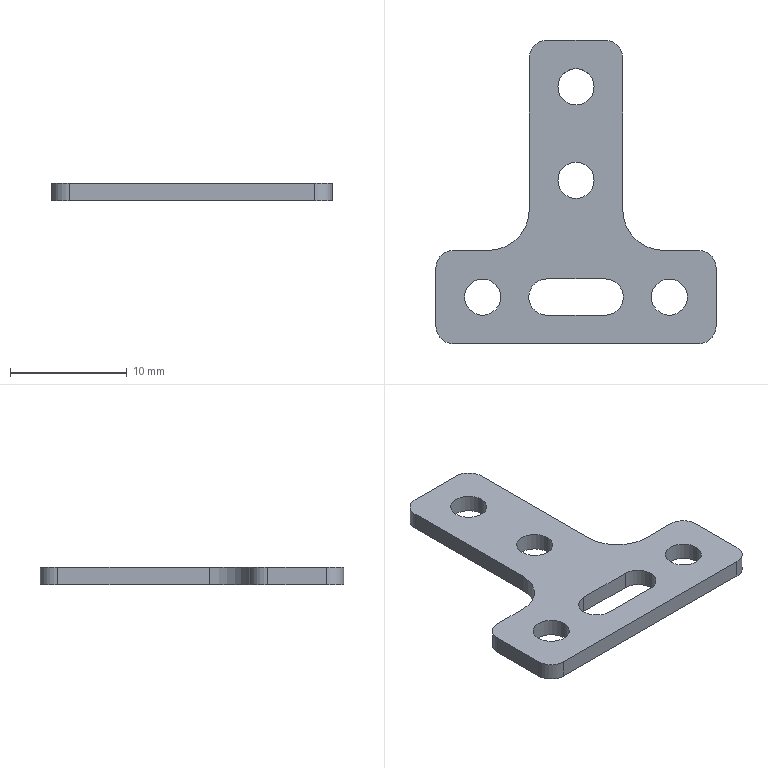Part | SolidWorks | features Fillet 2, Extrusion 1 | 1 solid | 31 faces | box 24 x 26 x 1.5 mm | volume 427.683 mm3 | cylinder 19 | plane 12 | commonest cylinder face diameters 3.1 x11 3 x6 7 x2
STEP:
#1=CARTESIAN_POINT('',(-6.45,0.,1.5));
#2=VERTEX_POINT('',#1);
#3=CARTESIAN_POINT('',(-9.55,0.,1.5));
#4=VERTEX_POINT('',#3);
#5=CARTESIAN_POINT('',(-8.,0.,1.5));
#6=DIRECTION('',(0.,0.,-1.));
#7=DIRECTION('',(1.,0.,0.));
#8=AXIS2_PLACEMENT_3D('',#5,#6,#7);
#9=CIRCLE('',#8,1.55);
#10=EDGE_CURVE('',#2,#4,#9,.T.);
#11=ORIENTED_EDGE('',*,*,#10,.F.);
#12=CARTESIAN_POINT('',(-6.45,0.,0.));
#13=VERTEX_POINT('',#12);
#14=CARTESIAN_POINT('',(-6.45,0.,1.5));
#15=DIRECTION('',(0.,0.,-1.));
#16=VECTOR('',#15,1000.);
#17=LINE('',#14,#16);
#18=EDGE_CURVE('',#2,#13,#17,.T.);
#19=ORIENTED_EDGE('',*,*,#18,.T.);
#20=CARTESIAN_POINT('',(-9.55,0.,0.));
#21=VERTEX_POINT('',#20);
#22=CARTESIAN_POINT('',(-8.,0.,0.));
#23=DIRECTION('',(0.,0.,-1.));
#24=DIRECTION('',(1.,0.,0.));
#25=AXIS2_PLACEMENT_3D('',#22,#23,#24);
#26=CIRCLE('',#25,1.55);
#27=EDGE_CURVE('',#13,#21,#26,.T.);
#28=ORIENTED_EDGE('',*,*,#27,.T.);
#29=CARTESIAN_POINT('',(-9.55,0.,1.5));
#30=DIRECTION('',(0.,0.,-1.));
#31=VECTOR('',#30,1000.);
#32=LINE('',#29,#31);
#33=EDGE_CURVE('',#4,#21,#32,.T.);
#34=ORIENTED_EDGE('',*,*,#33,.F.);
#35=EDGE_LOOP('',(#11,#19,#28,#34));
#36=FACE_OUTER_BOUND('',#35,.T.);
#37=CARTESIAN_POINT('',(-8.,0.,1.5));
#38=DIRECTION('',(0.,0.,-1.));
#39=DIRECTION('',(-1.,0.,0.));
#40=AXIS2_PLACEMENT_3D('',#37,#38,#39);
#41=CYLINDRICAL_SURFACE('',#40,1.55);
#42=ADVANCED_FACE('',(#36),#41,.F.);
#43=CARTESIAN_POINT('',(-1.55,18.,1.5));
#44=VERTEX_POINT('',#43);
#45=CARTESIAN_POINT('',(1.55,18.,1.5));
#46=VERTEX_POINT('',#45);
#47=CARTESIAN_POINT('',(0.,18.,1.5));
#48=DIRECTION('',(0.,0.,1.));
#49=DIRECTION('',(1.,0.,0.));
#50=AXIS2_PLACEMENT_3D('',#47,#48,#49);
#51=CIRCLE('',#50,1.55);
#52=EDGE_CURVE('',#44,#46,#51,.T.);
#53=ORIENTED_EDGE('',*,*,#52,.T.);
#54=CARTESIAN_POINT('',(1.55,18.,0.));
#55=VERTEX_POINT('',#54);
#56=CARTESIAN_POINT('',(1.55,18.,1.5));
#57=DIRECTION('',(0.,0.,-1.));
#58=VECTOR('',#57,1000.);
#59=LINE('',#56,#58);
#60=EDGE_CURVE('',#46,#55,#59,.T.);
#61=ORIENTED_EDGE('',*,*,#60,.T.);
#62=CARTESIAN_POINT('',(-1.55,18.,0.));
#63=VERTEX_POINT('',#62);
#64=CARTESIAN_POINT('',(0.,18.,0.));
#65=DIRECTION('',(0.,0.,1.));
#66=DIRECTION('',(1.,0.,0.));
#67=AXIS2_PLACEMENT_3D('',#64,#65,#66);
#68=CIRCLE('',#67,1.55);
#69=EDGE_CURVE('',#63,#55,#68,.T.);
#70=ORIENTED_EDGE('',*,*,#69,.F.);
#71=CARTESIAN_POINT('',(-1.55,18.,1.5));
#72=DIRECTION('',(0.,0.,-1.));
#73=VECTOR('',#72,1000.);
#74=LINE('',#71,#73);
#75=EDGE_CURVE('',#44,#63,#74,.T.);
#76=ORIENTED_EDGE('',*,*,#75,.F.);
#77=EDGE_LOOP('',(#53,#61,#70,#76));
#78=FACE_OUTER_BOUND('',#77,.T.);
#79=CARTESIAN_POINT('',(0.,18.,1.5));
#80=DIRECTION('',(0.,0.,-1.));
#81=DIRECTION('',(-1.,0.,0.));
#82=AXIS2_PLACEMENT_3D('',#79,#80,#81);
#83=CYLINDRICAL_SURFACE('',#82,1.55);
#84=ADVANCED_FACE('',(#78),#83,.F.);
#85=CARTESIAN_POINT('',(-1.55,10.,1.5));
#86=VERTEX_POINT('',#85);
#87=CARTESIAN_POINT('',(1.55,10.,1.5));
#88=VERTEX_POINT('',#87);
#89=CARTESIAN_POINT('',(0.,10.,1.5));
#90=DIRECTION('',(0.,0.,1.));
#91=DIRECTION('',(1.,0.,0.));
#92=AXIS2_PLACEMENT_3D('',#89,#90,#91);
#93=CIRCLE('',#92,1.55);
#94=EDGE_CURVE('',#86,#88,#93,.T.);
#95=ORIENTED_EDGE('',*,*,#94,.T.);
#96=CARTESIAN_POINT('',(1.55,10.,0.));
#97=VERTEX_POINT('',#96);
#98=CARTESIAN_POINT('',(1.55,10.,1.5));
#99=DIRECTION('',(0.,0.,-1.));
#100=VECTOR('',#99,1000.);
#101=LINE('',#98,#100);
#102=EDGE_CURVE('',#88,#97,#101,.T.);
#103=ORIENTED_EDGE('',*,*,#102,.T.);
#104=CARTESIAN_POINT('',(-1.55,10.,0.));
#105=VERTEX_POINT('',#104);
#106=CARTESIAN_POINT('',(0.,10.,0.));
#107=DIRECTION('',(0.,0.,1.));
#108=DIRECTION('',(1.,0.,0.));
#109=AXIS2_PLACEMENT_3D('',#106,#107,#108);
#110=CIRCLE('',#109,1.55);
#111=EDGE_CURVE('',#105,#97,#110,.T.);
#112=ORIENTED_EDGE('',*,*,#111,.F.);
#113=CARTESIAN_POINT('',(-1.55,10.,1.5));
#114=DIRECTION('',(0.,0.,-1.));
#115=VECTOR('',#114,1000.);
#116=LINE('',#113,#115);
#117=EDGE_CURVE('',#86,#105,#116,.T.);
#118=ORIENTED_EDGE('',*,*,#117,.F.);
#119=EDGE_LOOP('',(#95,#103,#112,#118));
#120=FACE_OUTER_BOUND('',#119,.T.);
#121=CARTESIAN_POINT('',(0.,10.,1.5));
#122=DIRECTION('',(0.,0.,-1.));
#123=DIRECTION('',(-1.,0.,0.));
#124=AXIS2_PLACEMENT_3D('',#121,#122,#123);
#125=CYLINDRICAL_SURFACE('',#124,1.55);
#126=ADVANCED_FACE('',(#120),#125,.F.);
#127=CARTESIAN_POINT('',(6.45,0.,1.5));
#128=VERTEX_POINT('',#127);
#129=CARTESIAN_POINT('',(9.55,0.,1.5));
#130=VERTEX_POINT('',#129);
#131=CARTESIAN_POINT('',(8.,0.,1.5));
#132=DIRECTION('',(0.,0.,1.));
#133=DIRECTION('',(1.,0.,0.));
#134=AXIS2_PLACEMENT_3D('',#131,#132,#133);
#135=CIRCLE('',#134,1.55);
#136=EDGE_CURVE('',#128,#130,#135,.T.);
#137=ORIENTED_EDGE('',*,*,#136,.T.);
#138=CARTESIAN_POINT('',(9.55,0.,0.));
#139=VERTEX_POINT('',#138);
#140=CARTESIAN_POINT('',(9.55,0.,1.5));
#141=DIRECTION('',(0.,0.,-1.));
#142=VECTOR('',#141,1000.);
#143=LINE('',#140,#142);
#144=EDGE_CURVE('',#130,#139,#143,.T.);
#145=ORIENTED_EDGE('',*,*,#144,.T.);
#146=CARTESIAN_POINT('',(6.45,0.,0.));
#147=VERTEX_POINT('',#146);
#148=CARTESIAN_POINT('',(8.,0.,0.));
#149=DIRECTION('',(0.,0.,1.));
#150=DIRECTION('',(1.,0.,0.));
#151=AXIS2_PLACEMENT_3D('',#148,#149,#150);
#152=CIRCLE('',#151,1.55);
#153=EDGE_CURVE('',#147,#139,#152,.T.);
#154=ORIENTED_EDGE('',*,*,#153,.F.);
#155=CARTESIAN_POINT('',(6.45,0.,1.5));
#156=DIRECTION('',(0.,0.,-1.));
#157=VECTOR('',#156,1000.);
#158=LINE('',#155,#157);
#159=EDGE_CURVE('',#128,#147,#158,.T.);
#160=ORIENTED_EDGE('',*,*,#159,.F.);
#161=EDGE_LOOP('',(#137,#145,#154,#160));
#162=FACE_OUTER_BOUND('',#161,.T.);
#163=CARTESIAN_POINT('',(8.,0.,1.5));
#164=DIRECTION('',(0.,0.,-1.));
#165=DIRECTION('',(-1.,0.,0.));
#166=AXIS2_PLACEMENT_3D('',#163,#164,#165);
#167=CYLINDRICAL_SURFACE('',#166,1.55);
#168=ADVANCED_FACE('',(#162),#167,.F.);
#169=CARTESIAN_POINT('',(-2.5,1.55,1.5));
#170=VERTEX_POINT('',#169);
#171=CARTESIAN_POINT('',(-4.05,0.,1.5));
#172=VERTEX_POINT('',#171);
#173=CARTESIAN_POINT('',(-2.5,0.,1.5));
#174=DIRECTION('',(0.,0.,1.));
#175=DIRECTION('',(1.,0.,0.));
#176=AXIS2_PLACEMENT_3D('',#173,#174,#175);
#177=CIRCLE('',#176,1.55);
#178=EDGE_CURVE('',#170,#172,#177,.T.);
#179=ORIENTED_EDGE('',*,*,#178,.T.);
#180=CARTESIAN_POINT('',(-4.05,0.,0.));
#181=VERTEX_POINT('',#180);
#182=CARTESIAN_POINT('',(-4.05,0.,1.5));
#183=DIRECTION('',(0.,0.,-1.));
#184=VECTOR('',#183,1000.);
#185=LINE('',#182,#184);
#186=EDGE_CURVE('',#172,#181,#185,.T.);
#187=ORIENTED_EDGE('',*,*,#186,.T.);
#188=CARTESIAN_POINT('',(-2.5,1.55,0.));
#189=VERTEX_POINT('',#188);
#190=CARTESIAN_POINT('',(-2.5,0.,0.));
#191=DIRECTION('',(0.,0.,1.));
#192=DIRECTION('',(1.,0.,0.));
#193=AXIS2_PLACEMENT_3D('',#190,#191,#192);
#194=CIRCLE('',#193,1.55);
#195=EDGE_CURVE('',#189,#181,#194,.T.);
#196=ORIENTED_EDGE('',*,*,#195,.F.);
#197=CARTESIAN_POINT('',(-2.5,1.55,1.5));
#198=DIRECTION('',(0.,0.,-1.));
#199=VECTOR('',#198,1000.);
#200=LINE('',#197,#199);
#201=EDGE_CURVE('',#170,#189,#200,.T.);
#202=ORIENTED_EDGE('',*,*,#201,.F.);
#203=EDGE_LOOP('',(#179,#187,#196,#202));
#204=FACE_OUTER_BOUND('',#203,.T.);
#205=CARTESIAN_POINT('',(-2.5,0.,1.5));
#206=DIRECTION('',(0.,0.,-1.));
#207=DIRECTION('',(-1.,0.,0.));
#208=AXIS2_PLACEMENT_3D('',#205,#206,#207);
#209=CYLINDRICAL_SURFACE('',#208,1.55);
#210=ADVANCED_FACE('',(#204),#209,.F.);
#211=CARTESIAN_POINT('',(4.,20.5,1.5));
#212=VERTEX_POINT('',#211);
#213=CARTESIAN_POINT('',(4.,7.5,1.5));
#214=VERTEX_POINT('',#213);
#215=CARTESIAN_POINT('',(4.,0.,1.5));
#216=DIRECTION('',(0.,-1.,0.));
#217=VECTOR('',#216,1000.);
#218=LINE('',#215,#217);
#219=EDGE_CURVE('',#212,#214,#218,.T.);
#220=ORIENTED_EDGE('',*,*,#219,.T.);
#221=CARTESIAN_POINT('',(4.,7.5,0.));
#222=VERTEX_POINT('',#221);
#223=CARTESIAN_POINT('',(4.,7.5,0.));
#224=DIRECTION('',(0.,0.,-1.));
#225=VECTOR('',#224,1000.);
#226=LINE('',#223,#225);
#227=EDGE_CURVE('',#214,#222,#226,.T.);
#228=ORIENTED_EDGE('',*,*,#227,.T.);
#229=CARTESIAN_POINT('',(4.,20.5,0.));
#230=VERTEX_POINT('',#229);
#231=CARTESIAN_POINT('',(4.,0.,0.));
#232=DIRECTION('',(0.,-1.,0.));
#233=VECTOR('',#232,1000.);
#234=LINE('',#231,#233);
#235=EDGE_CURVE('',#230,#222,#234,.T.);
#236=ORIENTED_EDGE('',*,*,#235,.F.);
#237=CARTESIAN_POINT('',(4.,20.5,1.5));
#238=DIRECTION('',(0.,0.,1.));
#239=VECTOR('',#238,1000.);
#240=LINE('',#237,#239);
#241=EDGE_CURVE('',#230,#212,#240,.T.);
#242=ORIENTED_EDGE('',*,*,#241,.T.);
#243=EDGE_LOOP('',(#220,#228,#236,#242));
#244=FACE_OUTER_BOUND('',#243,.T.);
#245=CARTESIAN_POINT('',(4.,0.,1.5));
#246=DIRECTION('',(1.,0.,0.));
#247=DIRECTION('',(0.,1.,0.));
#248=AXIS2_PLACEMENT_3D('',#245,#246,#247);
#249=PLANE('',#248);
#250=ADVANCED_FACE('',(#244),#249,.T.);
#251=CARTESIAN_POINT('',(2.5,22.,1.5));
#252=VERTEX_POINT('',#251);
#253=CARTESIAN_POINT('',(-2.5,22.,1.5));
#254=VERTEX_POINT('',#253);
#255=CARTESIAN_POINT('',(0.,22.,1.5));
#256=DIRECTION('',(-1.,0.,0.));
#257=VECTOR('',#256,1000.);
#258=LINE('',#255,#257);
#259=EDGE_CURVE('',#252,#254,#258,.T.);
#260=ORIENTED_EDGE('',*,*,#259,.F.);
#261=CARTESIAN_POINT('',(2.5,22.,0.));
#262=VERTEX_POINT('',#261);
#263=CARTESIAN_POINT('',(2.5,22.,0.));
#264=DIRECTION('',(0.,0.,-1.));
#265=VECTOR('',#264,1000.);
#266=LINE('',#263,#265);
#267=EDGE_CURVE('',#252,#262,#266,.T.);
#268=ORIENTED_EDGE('',*,*,#267,.T.);
#269=CARTESIAN_POINT('',(-2.5,22.,0.));
#270=VERTEX_POINT('',#269);
#271=CARTESIAN_POINT('',(0.,22.,0.));
#272=DIRECTION('',(-1.,0.,0.));
#273=VECTOR('',#272,1000.);
#274=LINE('',#271,#273);
#275=EDGE_CURVE('',#262,#270,#274,.T.);
#276=ORIENTED_EDGE('',*,*,#275,.T.);
#277=CARTESIAN_POINT('',(-2.5,22.,1.5));
#278=DIRECTION('',(0.,0.,1.));
#279=VECTOR('',#278,1000.);
#280=LINE('',#277,#279);
#281=EDGE_CURVE('',#270,#254,#280,.T.);
#282=ORIENTED_EDGE('',*,*,#281,.T.);
#283=EDGE_LOOP('',(#260,#268,#276,#282));
#284=FACE_OUTER_BOUND('',#283,.T.);
#285=CARTESIAN_POINT('',(0.,22.,1.5));
#286=DIRECTION('',(0.,-1.,0.));
#287=DIRECTION('',(0.,0.,-1.));
#288=AXIS2_PLACEMENT_3D('',#285,#286,#287);
#289=PLANE('',#288);
#290=ADVANCED_FACE('',(#284),#289,.F.);
#291=CARTESIAN_POINT('',(-4.,20.5,0.));
#292=VERTEX_POINT('',#291);
#293=CARTESIAN_POINT('',(-4.,7.5,0.));
#294=VERTEX_POINT('',#293);
#295=CARTESIAN_POINT('',(-4.,0.,0.));
#296=DIRECTION('',(0.,-1.,0.));
#297=VECTOR('',#296,1000.);
#298=LINE('',#295,#297);
#299=EDGE_CURVE('',#292,#294,#298,.T.);
#300=ORIENTED_EDGE('',*,*,#299,.T.);
#301=CARTESIAN_POINT('',(-4.,7.5,1.5));
#302=VERTEX_POINT('',#301);
#303=CARTESIAN_POINT('',(-4.,7.5,1.5));
#304=DIRECTION('',(0.,0.,1.));
#305=VECTOR('',#304,1000.);
#306=LINE('',#303,#305);
#307=EDGE_CURVE('',#294,#302,#306,.T.);
#308=ORIENTED_EDGE('',*,*,#307,.T.);
#309=CARTESIAN_POINT('',(-4.,20.5,1.5));
#310=VERTEX_POINT('',#309);
#311=CARTESIAN_POINT('',(-4.,0.,1.5));
#312=DIRECTION('',(0.,-1.,0.));
#313=VECTOR('',#312,1000.);
#314=LINE('',#311,#313);
#315=EDGE_CURVE('',#310,#302,#314,.T.);
#316=ORIENTED_EDGE('',*,*,#315,.F.);
#317=CARTESIAN_POINT('',(-4.,20.5,1.5));
#318=DIRECTION('',(0.,0.,-1.));
#319=VECTOR('',#318,1000.);
#320=LINE('',#317,#319);
#321=EDGE_CURVE('',#310,#292,#320,.T.);
#322=ORIENTED_EDGE('',*,*,#321,.T.);
#323=EDGE_LOOP('',(#300,#308,#316,#322));
#324=FACE_OUTER_BOUND('',#323,.T.);
#325=CARTESIAN_POINT('',(-4.,0.,1.5));
#326=DIRECTION('',(1.,0.,0.));
#327=DIRECTION('',(0.,1.,0.));
#328=AXIS2_PLACEMENT_3D('',#325,#326,#327);
#329=PLANE('',#328);
#330=ADVANCED_FACE('',(#324),#329,.F.);
#331=CARTESIAN_POINT('',(-7.5,4.,1.5));
#332=VERTEX_POINT('',#331);
#333=CARTESIAN_POINT('',(-10.5,4.,1.5));
#334=VERTEX_POINT('',#333);
#335=CARTESIAN_POINT('',(0.,4.,1.5));
#336=DIRECTION('',(-1.,0.,0.));
#337=VECTOR('',#336,1000.);
#338=LINE('',#335,#337);
#339=EDGE_CURVE('',#332,#334,#338,.T.);
#340=ORIENTED_EDGE('',*,*,#339,.F.);
#341=CARTESIAN_POINT('',(-7.5,4.,0.));
#342=VERTEX_POINT('',#341);
#343=CARTESIAN_POINT('',(-7.5,4.,0.));
#344=DIRECTION('',(0.,0.,-1.));
#345=VECTOR('',#344,1000.);
#346=LINE('',#343,#345);
#347=EDGE_CURVE('',#332,#342,#346,.T.);
#348=ORIENTED_EDGE('',*,*,#347,.T.);
#349=CARTESIAN_POINT('',(-10.5,4.,0.));
#350=VERTEX_POINT('',#349);
#351=CARTESIAN_POINT('',(0.,4.,0.));
#352=DIRECTION('',(-1.,0.,0.));
#353=VECTOR('',#352,1000.);
#354=LINE('',#351,#353);
#355=EDGE_CURVE('',#342,#350,#354,.T.);
#356=ORIENTED_EDGE('',*,*,#355,.T.);
#357=CARTESIAN_POINT('',(-10.5,4.,1.5));
#358=DIRECTION('',(0.,0.,1.));
#359=VECTOR('',#358,1000.);
#360=LINE('',#357,#359);
#361=EDGE_CURVE('',#350,#334,#360,.T.);
#362=ORIENTED_EDGE('',*,*,#361,.T.);
#363=EDGE_LOOP('',(#340,#348,#356,#362));
#364=FACE_OUTER_BOUND('',#363,.T.);
#365=CARTESIAN_POINT('',(0.,4.,1.5));
#366=DIRECTION('',(0.,-1.,0.));
#367=DIRECTION('',(1.,0.,0.));
#368=AXIS2_PLACEMENT_3D('',#365,#366,#367);
#369=PLANE('',#368);
#370=ADVANCED_FACE('',(#364),#369,.F.);
#371=CARTESIAN_POINT('',(-12.,2.5,0.));
#372=VERTEX_POINT('',#371);
#373=CARTESIAN_POINT('',(-12.,-2.5,0.));
#374=VERTEX_POINT('',#373);
#375=CARTESIAN_POINT('',(-12.,0.,0.));
#376=DIRECTION('',(0.,-1.,0.));
#377=VECTOR('',#376,1000.);
#378=LINE('',#375,#377);
#379=EDGE_CURVE('',#372,#374,#378,.T.);
#380=ORIENTED_EDGE('',*,*,#379,.T.);
#381=CARTESIAN_POINT('',(-12.,-2.5,1.5));
#382=VERTEX_POINT('',#381);
#383=CARTESIAN_POINT('',(-12.,-2.5,1.5));
#384=DIRECTION('',(0.,0.,1.));
#385=VECTOR('',#384,1000.);
#386=LINE('',#383,#385);
#387=EDGE_CURVE('',#374,#382,#386,.T.);
#388=ORIENTED_EDGE('',*,*,#387,.T.);
#389=CARTESIAN_POINT('',(-12.,2.5,1.5));
#390=VERTEX_POINT('',#389);
#391=CARTESIAN_POINT('',(-12.,0.,1.5));
#392=DIRECTION('',(0.,-1.,0.));
#393=VECTOR('',#392,1000.);
#394=LINE('',#391,#393);
#395=EDGE_CURVE('',#390,#382,#394,.T.);
#396=ORIENTED_EDGE('',*,*,#395,.F.);
#397=CARTESIAN_POINT('',(-12.,2.5,1.5));
#398=DIRECTION('',(0.,0.,-1.));
#399=VECTOR('',#398,1000.);
#400=LINE('',#397,#399);
#401=EDGE_CURVE('',#390,#372,#400,.T.);
#402=ORIENTED_EDGE('',*,*,#401,.T.);
#403=EDGE_LOOP('',(#380,#388,#396,#402));
#404=FACE_OUTER_BOUND('',#403,.T.);
#405=CARTESIAN_POINT('',(-12.,0.,1.5));
#406=DIRECTION('',(1.,0.,0.));
#407=DIRECTION('',(0.,0.,-1.));
#408=AXIS2_PLACEMENT_3D('',#405,#406,#407);
#409=PLANE('',#408);
#410=ADVANCED_FACE('',(#404),#409,.F.);
#411=CARTESIAN_POINT('',(-10.5,-4.,0.));
#412=VERTEX_POINT('',#411);
#413=CARTESIAN_POINT('',(10.5,-4.,0.));
#414=VERTEX_POINT('',#413);
#415=CARTESIAN_POINT('',(0.,-4.,0.));
#416=DIRECTION('',(1.,0.,0.));
#417=VECTOR('',#416,1000.);
#418=LINE('',#415,#417);
#419=EDGE_CURVE('',#412,#414,#418,.T.);
#420=ORIENTED_EDGE('',*,*,#419,.T.);
#421=CARTESIAN_POINT('',(10.5,-4.,1.5));
#422=VERTEX_POINT('',#421);
#423=CARTESIAN_POINT('',(10.5,-4.,1.5));
#424=DIRECTION('',(0.,0.,1.));
#425=VECTOR('',#424,1000.);
#426=LINE('',#423,#425);
#427=EDGE_CURVE('',#414,#422,#426,.T.);
#428=ORIENTED_EDGE('',*,*,#427,.T.);
#429=CARTESIAN_POINT('',(-10.5,-4.,1.5));
#430=VERTEX_POINT('',#429);
#431=CARTESIAN_POINT('',(0.,-4.,1.5));
#432=DIRECTION('',(1.,0.,0.));
#433=VECTOR('',#432,1000.);
#434=LINE('',#431,#433);
#435=EDGE_CURVE('',#430,#422,#434,.T.);
#436=ORIENTED_EDGE('',*,*,#435,.F.);
#437=CARTESIAN_POINT('',(-10.5,-4.,1.5));
#438=DIRECTION('',(0.,0.,-1.));
#439=VECTOR('',#438,1000.);
#440=LINE('',#437,#439);
#441=EDGE_CURVE('',#430,#412,#440,.T.);
#442=ORIENTED_EDGE('',*,*,#441,.T.);
#443=EDGE_LOOP('',(#420,#428,#436,#442));
#444=FACE_OUTER_BOUND('',#443,.T.);
#445=CARTESIAN_POINT('',(0.,-4.,1.5));
#446=DIRECTION('',(0.,1.,0.));
#447=DIRECTION('',(0.,0.,1.));
#448=AXIS2_PLACEMENT_3D('',#445,#446,#447);
#449=PLANE('',#448);
#450=ADVANCED_FACE('',(#444),#449,.F.);
#451=CARTESIAN_POINT('',(12.,2.5,0.));
#452=VERTEX_POINT('',#451);
#453=CARTESIAN_POINT('',(12.,-2.5,0.));
#454=VERTEX_POINT('',#453);
#455=CARTESIAN_POINT('',(12.,0.,0.));
#456=DIRECTION('',(0.,-1.,0.));
#457=VECTOR('',#456,1000.);
#458=LINE('',#455,#457);
#459=EDGE_CURVE('',#452,#454,#458,.T.);
#460=ORIENTED_EDGE('',*,*,#459,.F.);
#461=CARTESIAN_POINT('',(12.,2.5,1.5));
#462=VERTEX_POINT('',#461);
#463=CARTESIAN_POINT('',(12.,2.5,1.5));
#464=DIRECTION('',(0.,0.,1.));
#465=VECTOR('',#464,1000.);
#466=LINE('',#463,#465);
#467=EDGE_CURVE('',#452,#462,#466,.T.);
#468=ORIENTED_EDGE('',*,*,#467,.T.);
#469=CARTESIAN_POINT('',(12.,-2.5,1.5));
#470=VERTEX_POINT('',#469);
#471=CARTESIAN_POINT('',(12.,0.,1.5));
#472=DIRECTION('',(0.,-1.,0.));
#473=VECTOR('',#472,1000.);
#474=LINE('',#471,#473);
#475=EDGE_CURVE('',#462,#470,#474,.T.);
#476=ORIENTED_EDGE('',*,*,#475,.T.);
#477=CARTESIAN_POINT('',(12.,-2.5,0.));
#478=DIRECTION('',(0.,0.,-1.));
#479=VECTOR('',#478,1000.);
#480=LINE('',#477,#479);
#481=EDGE_CURVE('',#470,#454,#480,.T.);
#482=ORIENTED_EDGE('',*,*,#481,.T.);
#483=EDGE_LOOP('',(#460,#468,#476,#482));
#484=FACE_OUTER_BOUND('',#483,.T.);
#485=CARTESIAN_POINT('',(12.,0.,1.5));
#486=DIRECTION('',(1.,0.,0.));
#487=DIRECTION('',(0.,0.,-1.));
#488=AXIS2_PLACEMENT_3D('',#485,#486,#487);
#489=PLANE('',#488);
#490=ADVANCED_FACE('',(#484),#489,.T.);
#491=CARTESIAN_POINT('',(2.5,-1.55,0.));
#492=VERTEX_POINT('',#491);
#493=CARTESIAN_POINT('',(2.5,1.55,0.));
#494=VERTEX_POINT('',#493);
#495=CARTESIAN_POINT('',(2.5,0.,0.));
#496=DIRECTION('',(0.,0.,1.));
#497=DIRECTION('',(1.,0.,0.));
#498=AXIS2_PLACEMENT_3D('',#495,#496,#497);
#499=CIRCLE('',#498,1.55);
#500=EDGE_CURVE('',#492,#494,#499,.T.);
#501=ORIENTED_EDGE('',*,*,#500,.F.);
#502=CARTESIAN_POINT('',(2.5,-1.55,1.5));
#503=VERTEX_POINT('',#502);
#504=CARTESIAN_POINT('',(2.5,-1.55,1.5));
#505=DIRECTION('',(0.,0.,-1.));
#506=VECTOR('',#505,1000.);
#507=LINE('',#504,#506);
#508=EDGE_CURVE('',#503,#492,#507,.T.);
#509=ORIENTED_EDGE('',*,*,#508,.F.);
#510=CARTESIAN_POINT('',(2.5,1.55,1.5));
#511=VERTEX_POINT('',#510);
#512=CARTESIAN_POINT('',(2.5,0.,1.5));
#513=DIRECTION('',(0.,0.,1.));
#514=DIRECTION('',(1.,0.,0.));
#515=AXIS2_PLACEMENT_3D('',#512,#513,#514);
#516=CIRCLE('',#515,1.55);
#517=EDGE_CURVE('',#503,#511,#516,.T.);
#518=ORIENTED_EDGE('',*,*,#517,.T.);
#519=CARTESIAN_POINT('',(2.5,1.55,1.5));
#520=DIRECTION('',(0.,0.,-1.));
#521=VECTOR('',#520,1000.);
#522=LINE('',#519,#521);
#523=EDGE_CURVE('',#511,#494,#522,.T.);
#524=ORIENTED_EDGE('',*,*,#523,.T.);
#525=EDGE_LOOP('',(#501,#509,#518,#524));
#526=FACE_OUTER_BOUND('',#525,.T.);
#527=CARTESIAN_POINT('',(2.5,0.,1.5));
#528=DIRECTION('',(0.,0.,-1.));
#529=DIRECTION('',(-1.,0.,0.));
#530=AXIS2_PLACEMENT_3D('',#527,#528,#529);
#531=CYLINDRICAL_SURFACE('',#530,1.55);
#532=ADVANCED_FACE('',(#526),#531,.F.);
#533=CARTESIAN_POINT('',(-2.5,-1.55,0.));
#534=VERTEX_POINT('',#533);
#535=CARTESIAN_POINT('',(0.,-1.55,0.));
#536=DIRECTION('',(1.,0.,0.));
#537=VECTOR('',#536,1000.);
#538=LINE('',#535,#537);
#539=EDGE_CURVE('',#534,#492,#538,.T.);
#540=ORIENTED_EDGE('',*,*,#539,.F.);
#541=CARTESIAN_POINT('',(-2.5,-1.55,1.5));
#542=VERTEX_POINT('',#541);
#543=CARTESIAN_POINT('',(-2.5,-1.55,1.5));
#544=DIRECTION('',(0.,0.,-1.));
#545=VECTOR('',#544,1000.);
#546=LINE('',#543,#545);
#547=EDGE_CURVE('',#542,#534,#546,.T.);
#548=ORIENTED_EDGE('',*,*,#547,.F.);
#549=CARTESIAN_POINT('',(0.,-1.55,1.5));
#550=DIRECTION('',(1.,0.,0.));
#551=VECTOR('',#550,1000.);
#552=LINE('',#549,#551);
#553=EDGE_CURVE('',#542,#503,#552,.T.);
#554=ORIENTED_EDGE('',*,*,#553,.T.);
#555=ORIENTED_EDGE('',*,*,#508,.T.);
#556=EDGE_LOOP('',(#540,#548,#554,#555));
#557=FACE_OUTER_BOUND('',#556,.T.);
#558=CARTESIAN_POINT('',(0.,-1.55,1.5));
#559=DIRECTION('',(0.,1.,0.));
#560=DIRECTION('',(-1.,0.,0.));
#561=AXIS2_PLACEMENT_3D('',#558,#559,#560);
#562=PLANE('',#561);
#563=ADVANCED_FACE('',(#557),#562,.T.);
#564=ORIENTED_EDGE('',*,*,#186,.F.);
#565=CARTESIAN_POINT('',(-2.5,0.,1.5));
#566=DIRECTION('',(0.,0.,1.));
#567=DIRECTION('',(1.,0.,0.));
#568=AXIS2_PLACEMENT_3D('',#565,#566,#567);
#569=CIRCLE('',#568,1.55);
#570=EDGE_CURVE('',#172,#542,#569,.T.);
#571=ORIENTED_EDGE('',*,*,#570,.T.);
#572=ORIENTED_EDGE('',*,*,#547,.T.);
#573=CARTESIAN_POINT('',(-2.5,0.,0.));
#574=DIRECTION('',(0.,0.,1.));
#575=DIRECTION('',(1.,0.,0.));
#576=AXIS2_PLACEMENT_3D('',#573,#574,#575);
#577=CIRCLE('',#576,1.55);
#578=EDGE_CURVE('',#181,#534,#577,.T.);
#579=ORIENTED_EDGE('',*,*,#578,.F.);
#580=EDGE_LOOP('',(#564,#571,#572,#579));
#581=FACE_OUTER_BOUND('',#580,.T.);
#582=CARTESIAN_POINT('',(-2.5,0.,1.5));
#583=DIRECTION('',(0.,0.,-1.));
#584=DIRECTION('',(-1.,0.,0.));
#585=AXIS2_PLACEMENT_3D('',#582,#583,#584);
#586=CYLINDRICAL_SURFACE('',#585,1.55);
#587=ADVANCED_FACE('',(#581),#586,.F.);
#588=ORIENTED_EDGE('',*,*,#144,.F.);
#589=CARTESIAN_POINT('',(8.,0.,1.5));
#590=DIRECTION('',(0.,0.,1.));
#591=DIRECTION('',(1.,0.,0.));
#592=AXIS2_PLACEMENT_3D('',#589,#590,#591);
#593=CIRCLE('',#592,1.55);
#594=EDGE_CURVE('',#130,#128,#593,.T.);
#595=ORIENTED_EDGE('',*,*,#594,.T.);
#596=ORIENTED_EDGE('',*,*,#159,.T.);
#597=CARTESIAN_POINT('',(8.,0.,0.));
#598=DIRECTION('',(0.,0.,1.));
#599=DIRECTION('',(1.,0.,0.));
#600=AXIS2_PLACEMENT_3D('',#597,#598,#599);
#601=CIRCLE('',#600,1.55);
#602=EDGE_CURVE('',#139,#147,#601,.T.);
#603=ORIENTED_EDGE('',*,*,#602,.F.);
#604=EDGE_LOOP('',(#588,#595,#596,#603));
#605=FACE_OUTER_BOUND('',#604,.T.);
#606=CARTESIAN_POINT('',(8.,0.,1.5));
#607=DIRECTION('',(0.,0.,-1.));
#608=DIRECTION('',(-1.,0.,0.));
#609=AXIS2_PLACEMENT_3D('',#606,#607,#608);
#610=CYLINDRICAL_SURFACE('',#609,1.55);
#611=ADVANCED_FACE('',(#605),#610,.F.);
#612=ORIENTED_EDGE('',*,*,#102,.F.);
#613=CARTESIAN_POINT('',(0.,10.,1.5));
#614=DIRECTION('',(0.,0.,1.));
#615=DIRECTION('',(1.,0.,0.));
#616=AXIS2_PLACEMENT_3D('',#613,#614,#615);
#617=CIRCLE('',#616,1.55);
#618=EDGE_CURVE('',#88,#86,#617,.T.);
#619=ORIENTED_EDGE('',*,*,#618,.T.);
#620=ORIENTED_EDGE('',*,*,#117,.T.);
#621=CARTESIAN_POINT('',(0.,10.,0.));
#622=DIRECTION('',(0.,0.,1.));
#623=DIRECTION('',(1.,0.,0.));
#624=AXIS2_PLACEMENT_3D('',#621,#622,#623);
#625=CIRCLE('',#624,1.55);
#626=EDGE_CURVE('',#97,#105,#625,.T.);
#627=ORIENTED_EDGE('',*,*,#626,.F.);
#628=EDGE_LOOP('',(#612,#619,#620,#627));
#629=FACE_OUTER_BOUND('',#628,.T.);
#630=CARTESIAN_POINT('',(0.,10.,1.5));
#631=DIRECTION('',(0.,0.,-1.));
#632=DIRECTION('',(-1.,0.,0.));
#633=AXIS2_PLACEMENT_3D('',#630,#631,#632);
#634=CYLINDRICAL_SURFACE('',#633,1.55);
#635=ADVANCED_FACE('',(#629),#634,.F.);
#636=ORIENTED_EDGE('',*,*,#60,.F.);
#637=CARTESIAN_POINT('',(0.,18.,1.5));
#638=DIRECTION('',(0.,0.,1.));
#639=DIRECTION('',(1.,0.,0.));
#640=AXIS2_PLACEMENT_3D('',#637,#638,#639);
#641=CIRCLE('',#640,1.55);
#642=EDGE_CURVE('',#46,#44,#641,.T.);
#643=ORIENTED_EDGE('',*,*,#642,.T.);
#644=ORIENTED_EDGE('',*,*,#75,.T.);
#645=CARTESIAN_POINT('',(0.,18.,0.));
#646=DIRECTION('',(0.,0.,1.));
#647=DIRECTION('',(1.,0.,0.));
#648=AXIS2_PLACEMENT_3D('',#645,#646,#647);
#649=CIRCLE('',#648,1.55);
#650=EDGE_CURVE('',#55,#63,#649,.T.);
#651=ORIENTED_EDGE('',*,*,#650,.F.);
#652=EDGE_LOOP('',(#636,#643,#644,#651));
#653=FACE_OUTER_BOUND('',#652,.T.);
#654=CARTESIAN_POINT('',(0.,18.,1.5));
#655=DIRECTION('',(0.,0.,-1.));
#656=DIRECTION('',(-1.,0.,0.));
#657=AXIS2_PLACEMENT_3D('',#654,#655,#656);
#658=CYLINDRICAL_SURFACE('',#657,1.55);
#659=ADVANCED_FACE('',(#653),#658,.F.);
#660=CARTESIAN_POINT('',(7.5,4.,0.));
#661=VERTEX_POINT('',#660);
#662=CARTESIAN_POINT('',(10.5,4.,0.));
#663=VERTEX_POINT('',#662);
#664=CARTESIAN_POINT('',(0.,4.,0.));
#665=DIRECTION('',(1.,0.,0.));
#666=VECTOR('',#665,1000.);
#667=LINE('',#664,#666);
#668=EDGE_CURVE('',#661,#663,#667,.T.);
#669=ORIENTED_EDGE('',*,*,#668,.F.);
#670=CARTESIAN_POINT('',(7.5,4.,1.5));
#671=VERTEX_POINT('',#670);
#672=CARTESIAN_POINT('',(7.5,4.,1.5));
#673=DIRECTION('',(0.,0.,1.));
#674=VECTOR('',#673,1000.);
#675=LINE('',#672,#674);
#676=EDGE_CURVE('',#661,#671,#675,.T.);
#677=ORIENTED_EDGE('',*,*,#676,.T.);
#678=CARTESIAN_POINT('',(10.5,4.,1.5));
#679=VERTEX_POINT('',#678);
#680=CARTESIAN_POINT('',(0.,4.,1.5));
#681=DIRECTION('',(1.,0.,0.));
#682=VECTOR('',#681,1000.);
#683=LINE('',#680,#682);
#684=EDGE_CURVE('',#671,#679,#683,.T.);
#685=ORIENTED_EDGE('',*,*,#684,.T.);
#686=CARTESIAN_POINT('',(10.5,4.,1.5));
#687=DIRECTION('',(0.,0.,-1.));
#688=VECTOR('',#687,1000.);
#689=LINE('',#686,#688);
#690=EDGE_CURVE('',#679,#663,#689,.T.);
#691=ORIENTED_EDGE('',*,*,#690,.T.);
#692=EDGE_LOOP('',(#669,#677,#685,#691));
#693=FACE_OUTER_BOUND('',#692,.T.);
#694=CARTESIAN_POINT('',(0.,4.,1.5));
#695=DIRECTION('',(0.,1.,0.));
#696=DIRECTION('',(-1.,0.,0.));
#697=AXIS2_PLACEMENT_3D('',#694,#695,#696);
#698=PLANE('',#697);
#699=ADVANCED_FACE('',(#693),#698,.T.);
#700=CARTESIAN_POINT('',(0.,1.55,0.));
#701=DIRECTION('',(1.,0.,0.));
#702=VECTOR('',#701,1000.);
#703=LINE('',#700,#702);
#704=EDGE_CURVE('',#189,#494,#703,.T.);
#705=ORIENTED_EDGE('',*,*,#704,.T.);
#706=ORIENTED_EDGE('',*,*,#523,.F.);
#707=CARTESIAN_POINT('',(0.,1.55,1.5));
#708=DIRECTION('',(1.,0.,0.));
#709=VECTOR('',#708,1000.);
#710=LINE('',#707,#709);
#711=EDGE_CURVE('',#170,#511,#710,.T.);
#712=ORIENTED_EDGE('',*,*,#711,.F.);
#713=ORIENTED_EDGE('',*,*,#201,.T.);
#714=EDGE_LOOP('',(#705,#706,#712,#713));
#715=FACE_OUTER_BOUND('',#714,.T.);
#716=CARTESIAN_POINT('',(0.,1.55,1.5));
#717=DIRECTION('',(0.,1.,0.));
#718=DIRECTION('',(-1.,0.,0.));
#719=AXIS2_PLACEMENT_3D('',#716,#717,#718);
#720=PLANE('',#719);
#721=ADVANCED_FACE('',(#715),#720,.F.);
#722=ORIENTED_EDGE('',*,*,#18,.F.);
#723=CARTESIAN_POINT('',(-8.,0.,1.5));
#724=DIRECTION('',(0.,0.,-1.));
#725=DIRECTION('',(1.,0.,0.));
#726=AXIS2_PLACEMENT_3D('',#723,#724,#725);
#727=CIRCLE('',#726,1.55);
#728=EDGE_CURVE('',#4,#2,#727,.T.);
#729=ORIENTED_EDGE('',*,*,#728,.F.);
#730=ORIENTED_EDGE('',*,*,#33,.T.);
#731=CARTESIAN_POINT('',(-8.,0.,0.));
#732=DIRECTION('',(0.,0.,-1.));
#733=DIRECTION('',(1.,0.,0.));
#734=AXIS2_PLACEMENT_3D('',#731,#732,#733);
#735=CIRCLE('',#734,1.55);
#736=EDGE_CURVE('',#21,#13,#735,.T.);
#737=ORIENTED_EDGE('',*,*,#736,.T.);
#738=EDGE_LOOP('',(#722,#729,#730,#737));
#739=FACE_OUTER_BOUND('',#738,.T.);
#740=CARTESIAN_POINT('',(-8.,0.,1.5));
#741=DIRECTION('',(0.,0.,-1.));
#742=DIRECTION('',(-1.,0.,0.));
#743=AXIS2_PLACEMENT_3D('',#740,#741,#742);
#744=CYLINDRICAL_SURFACE('',#743,1.55);
#745=ADVANCED_FACE('',(#739),#744,.F.);
#746=ORIENTED_EDGE('',*,*,#517,.F.);
#747=ORIENTED_EDGE('',*,*,#553,.F.);
#748=ORIENTED_EDGE('',*,*,#570,.F.);
#749=ORIENTED_EDGE('',*,*,#178,.F.);
#750=ORIENTED_EDGE('',*,*,#711,.T.);
#751=EDGE_LOOP('',(#746,#747,#748,#749,#750));
#752=FACE_BOUND('',#751,.T.);
#753=ORIENTED_EDGE('',*,*,#219,.F.);
#754=CARTESIAN_POINT('',(2.5,20.5,1.5));
#755=DIRECTION('',(0.,0.,1.));
#756=DIRECTION('',(1.,0.,0.));
#757=AXIS2_PLACEMENT_3D('',#754,#755,#756);
#758=CIRCLE('',#757,1.5);
#759=EDGE_CURVE('',#212,#252,#758,.T.);
#760=ORIENTED_EDGE('',*,*,#759,.T.);
#761=ORIENTED_EDGE('',*,*,#259,.T.);
#762=CARTESIAN_POINT('',(-2.5,20.5,1.5));
#763=DIRECTION('',(0.,0.,1.));
#764=DIRECTION('',(1.,0.,0.));
#765=AXIS2_PLACEMENT_3D('',#762,#763,#764);
#766=CIRCLE('',#765,1.5);
#767=EDGE_CURVE('',#254,#310,#766,.T.);
#768=ORIENTED_EDGE('',*,*,#767,.T.);
#769=ORIENTED_EDGE('',*,*,#315,.T.);
#770=CARTESIAN_POINT('',(-7.5,7.5,1.5));
#771=DIRECTION('',(0.,0.,-1.));
#772=DIRECTION('',(1.,0.,0.));
#773=AXIS2_PLACEMENT_3D('',#770,#771,#772);
#774=CIRCLE('',#773,3.5);
#775=EDGE_CURVE('',#302,#332,#774,.T.);
#776=ORIENTED_EDGE('',*,*,#775,.T.);
#777=ORIENTED_EDGE('',*,*,#339,.T.);
#778=CARTESIAN_POINT('',(-10.5,2.5,1.5));
#779=DIRECTION('',(0.,0.,1.));
#780=DIRECTION('',(1.,0.,0.));
#781=AXIS2_PLACEMENT_3D('',#778,#779,#780);
#782=CIRCLE('',#781,1.5);
#783=EDGE_CURVE('',#334,#390,#782,.T.);
#784=ORIENTED_EDGE('',*,*,#783,.T.);
#785=ORIENTED_EDGE('',*,*,#395,.T.);
#786=CARTESIAN_POINT('',(-10.5,-2.5,1.5));
#787=DIRECTION('',(0.,0.,1.));
#788=DIRECTION('',(1.,0.,0.));
#789=AXIS2_PLACEMENT_3D('',#786,#787,#788);
#790=CIRCLE('',#789,1.5);
#791=EDGE_CURVE('',#382,#430,#790,.T.);
#792=ORIENTED_EDGE('',*,*,#791,.T.);
#793=ORIENTED_EDGE('',*,*,#435,.T.);
#794=CARTESIAN_POINT('',(10.5,-2.5,1.5));
#795=DIRECTION('',(0.,0.,1.));
#796=DIRECTION('',(1.,0.,0.));
#797=AXIS2_PLACEMENT_3D('',#794,#795,#796);
#798=CIRCLE('',#797,1.5);
#799=EDGE_CURVE('',#422,#470,#798,.T.);
#800=ORIENTED_EDGE('',*,*,#799,.T.);
#801=ORIENTED_EDGE('',*,*,#475,.F.);
#802=CARTESIAN_POINT('',(10.5,2.5,1.5));
#803=DIRECTION('',(0.,0.,1.));
#804=DIRECTION('',(1.,0.,0.));
#805=AXIS2_PLACEMENT_3D('',#802,#803,#804);
#806=CIRCLE('',#805,1.5);
#807=EDGE_CURVE('',#462,#679,#806,.T.);
#808=ORIENTED_EDGE('',*,*,#807,.T.);
#809=ORIENTED_EDGE('',*,*,#684,.F.);
#810=CARTESIAN_POINT('',(7.5,7.5,1.5));
#811=DIRECTION('',(0.,0.,-1.));
#812=DIRECTION('',(1.,0.,0.));
#813=AXIS2_PLACEMENT_3D('',#810,#811,#812);
#814=CIRCLE('',#813,3.5);
#815=EDGE_CURVE('',#671,#214,#814,.T.);
#816=ORIENTED_EDGE('',*,*,#815,.T.);
#817=EDGE_LOOP('',(#753,#760,#761,#768,#769,#776,#777,#784,#785,#792,#793,#800,#801,#808,#809,#816));
#818=FACE_OUTER_BOUND('',#817,.T.);
#819=ORIENTED_EDGE('',*,*,#52,.F.);
#820=ORIENTED_EDGE('',*,*,#642,.F.);
#821=EDGE_LOOP('',(#819,#820));
#822=FACE_BOUND('',#821,.T.);
#823=ORIENTED_EDGE('',*,*,#94,.F.);
#824=ORIENTED_EDGE('',*,*,#618,.F.);
#825=EDGE_LOOP('',(#823,#824));
#826=FACE_BOUND('',#825,.T.);
#827=ORIENTED_EDGE('',*,*,#136,.F.);
#828=ORIENTED_EDGE('',*,*,#594,.F.);
#829=EDGE_LOOP('',(#827,#828));
#830=FACE_BOUND('',#829,.T.);
#831=ORIENTED_EDGE('',*,*,#728,.T.);
#832=ORIENTED_EDGE('',*,*,#10,.T.);
#833=EDGE_LOOP('',(#831,#832));
#834=FACE_BOUND('',#833,.T.);
#835=CARTESIAN_POINT('',(0.,0.,1.5));
#836=DIRECTION('',(0.,0.,1.));
#837=DIRECTION('',(1.,0.,0.));
#838=AXIS2_PLACEMENT_3D('',#835,#836,#837);
#839=PLANE('',#838);
#840=ADVANCED_FACE('',(#752,#818,#822,#826,#830,#834),#839,.T.);
#841=ORIENTED_EDGE('',*,*,#500,.T.);
#842=ORIENTED_EDGE('',*,*,#704,.F.);
#843=ORIENTED_EDGE('',*,*,#195,.T.);
#844=ORIENTED_EDGE('',*,*,#578,.T.);
#845=ORIENTED_EDGE('',*,*,#539,.T.);
#846=EDGE_LOOP('',(#841,#842,#843,#844,#845));
#847=FACE_BOUND('',#846,.T.);
#848=ORIENTED_EDGE('',*,*,#275,.F.);
#849=CARTESIAN_POINT('',(2.5,20.5,0.));
#850=DIRECTION('',(0.,0.,-1.));
#851=DIRECTION('',(1.,0.,0.));
#852=AXIS2_PLACEMENT_3D('',#849,#850,#851);
#853=CIRCLE('',#852,1.5);
#854=EDGE_CURVE('',#262,#230,#853,.T.);
#855=ORIENTED_EDGE('',*,*,#854,.T.);
#856=ORIENTED_EDGE('',*,*,#235,.T.);
#857=CARTESIAN_POINT('',(7.5,7.5,0.));
#858=DIRECTION('',(0.,0.,1.));
#859=DIRECTION('',(1.,0.,0.));
#860=AXIS2_PLACEMENT_3D('',#857,#858,#859);
#861=CIRCLE('',#860,3.5);
#862=EDGE_CURVE('',#222,#661,#861,.T.);
#863=ORIENTED_EDGE('',*,*,#862,.T.);
#864=ORIENTED_EDGE('',*,*,#668,.T.);
#865=CARTESIAN_POINT('',(10.5,2.5,0.));
#866=DIRECTION('',(0.,0.,-1.));
#867=DIRECTION('',(1.,0.,0.));
#868=AXIS2_PLACEMENT_3D('',#865,#866,#867);
#869=CIRCLE('',#868,1.5);
#870=EDGE_CURVE('',#663,#452,#869,.T.);
#871=ORIENTED_EDGE('',*,*,#870,.T.);
#872=ORIENTED_EDGE('',*,*,#459,.T.);
#873=CARTESIAN_POINT('',(10.5,-2.5,0.));
#874=DIRECTION('',(0.,0.,-1.));
#875=DIRECTION('',(1.,0.,0.));
#876=AXIS2_PLACEMENT_3D('',#873,#874,#875);
#877=CIRCLE('',#876,1.5);
#878=EDGE_CURVE('',#454,#414,#877,.T.);
#879=ORIENTED_EDGE('',*,*,#878,.T.);
#880=ORIENTED_EDGE('',*,*,#419,.F.);
#881=CARTESIAN_POINT('',(-10.5,-2.5,0.));
#882=DIRECTION('',(0.,0.,-1.));
#883=DIRECTION('',(1.,0.,0.));
#884=AXIS2_PLACEMENT_3D('',#881,#882,#883);
#885=CIRCLE('',#884,1.5);
#886=EDGE_CURVE('',#412,#374,#885,.T.);
#887=ORIENTED_EDGE('',*,*,#886,.T.);
#888=ORIENTED_EDGE('',*,*,#379,.F.);
#889=CARTESIAN_POINT('',(-10.5,2.5,0.));
#890=DIRECTION('',(0.,0.,-1.));
#891=DIRECTION('',(1.,0.,0.));
#892=AXIS2_PLACEMENT_3D('',#889,#890,#891);
#893=CIRCLE('',#892,1.5);
#894=EDGE_CURVE('',#372,#350,#893,.T.);
#895=ORIENTED_EDGE('',*,*,#894,.T.);
#896=ORIENTED_EDGE('',*,*,#355,.F.);
#897=CARTESIAN_POINT('',(-7.5,7.5,0.));
#898=DIRECTION('',(0.,0.,1.));
#899=DIRECTION('',(1.,0.,0.));
#900=AXIS2_PLACEMENT_3D('',#897,#898,#899);
#901=CIRCLE('',#900,3.5);
#902=EDGE_CURVE('',#342,#294,#901,.T.);
#903=ORIENTED_EDGE('',*,*,#902,.T.);
#904=ORIENTED_EDGE('',*,*,#299,.F.);
#905=CARTESIAN_POINT('',(-2.5,20.5,0.));
#906=DIRECTION('',(0.,0.,-1.));
#907=DIRECTION('',(1.,0.,0.));
#908=AXIS2_PLACEMENT_3D('',#905,#906,#907);
#909=CIRCLE('',#908,1.5);
#910=EDGE_CURVE('',#292,#270,#909,.T.);
#911=ORIENTED_EDGE('',*,*,#910,.T.);
#912=EDGE_LOOP('',(#848,#855,#856,#863,#864,#871,#872,#879,#880,#887,#888,#895,#896,#903,#904,#911));
#913=FACE_OUTER_BOUND('',#912,.T.);
#914=ORIENTED_EDGE('',*,*,#69,.T.);
#915=ORIENTED_EDGE('',*,*,#650,.T.);
#916=EDGE_LOOP('',(#914,#915));
#917=FACE_BOUND('',#916,.T.);
#918=ORIENTED_EDGE('',*,*,#111,.T.);
#919=ORIENTED_EDGE('',*,*,#626,.T.);
#920=EDGE_LOOP('',(#918,#919));
#921=FACE_BOUND('',#920,.T.);
#922=ORIENTED_EDGE('',*,*,#153,.T.);
#923=ORIENTED_EDGE('',*,*,#602,.T.);
#924=EDGE_LOOP('',(#922,#923));
#925=FACE_BOUND('',#924,.T.);
#926=ORIENTED_EDGE('',*,*,#736,.F.);
#927=ORIENTED_EDGE('',*,*,#27,.F.);
#928=EDGE_LOOP('',(#926,#927));
#929=FACE_BOUND('',#928,.T.);
#930=CARTESIAN_POINT('',(0.,0.,0.));
#931=DIRECTION('',(0.,0.,1.));
#932=DIRECTION('',(1.,0.,0.));
#933=AXIS2_PLACEMENT_3D('',#930,#931,#932);
#934=PLANE('',#933);
#935=ADVANCED_FACE('',(#847,#913,#917,#921,#925,#929),#934,.F.);
#936=ORIENTED_EDGE('',*,*,#759,.F.);
#937=ORIENTED_EDGE('',*,*,#241,.F.);
#938=ORIENTED_EDGE('',*,*,#854,.F.);
#939=ORIENTED_EDGE('',*,*,#267,.F.);
#940=EDGE_LOOP('',(#936,#937,#938,#939));
#941=FACE_OUTER_BOUND('',#940,.T.);
#942=CARTESIAN_POINT('',(2.5,20.5,1.5));
#943=DIRECTION('',(0.,0.,1.));
#944=DIRECTION('',(1.,0.,0.));
#945=AXIS2_PLACEMENT_3D('',#942,#943,#944);
#946=CYLINDRICAL_SURFACE('',#945,1.5);
#947=ADVANCED_FACE('',(#941),#946,.T.);
#948=ORIENTED_EDGE('',*,*,#767,.F.);
#949=ORIENTED_EDGE('',*,*,#281,.F.);
#950=ORIENTED_EDGE('',*,*,#910,.F.);
#951=ORIENTED_EDGE('',*,*,#321,.F.);
#952=EDGE_LOOP('',(#948,#949,#950,#951));
#953=FACE_OUTER_BOUND('',#952,.T.);
#954=CARTESIAN_POINT('',(-2.5,20.5,1.5));
#955=DIRECTION('',(0.,0.,-1.));
#956=DIRECTION('',(-1.,0.,0.));
#957=AXIS2_PLACEMENT_3D('',#954,#955,#956);
#958=CYLINDRICAL_SURFACE('',#957,1.5);
#959=ADVANCED_FACE('',(#953),#958,.T.);
#960=ORIENTED_EDGE('',*,*,#807,.F.);
#961=ORIENTED_EDGE('',*,*,#467,.F.);
#962=ORIENTED_EDGE('',*,*,#870,.F.);
#963=ORIENTED_EDGE('',*,*,#690,.F.);
#964=EDGE_LOOP('',(#960,#961,#962,#963));
#965=FACE_OUTER_BOUND('',#964,.T.);
#966=CARTESIAN_POINT('',(10.5,2.5,1.5));
#967=DIRECTION('',(0.,0.,-1.));
#968=DIRECTION('',(-1.,0.,0.));
#969=AXIS2_PLACEMENT_3D('',#966,#967,#968);
#970=CYLINDRICAL_SURFACE('',#969,1.5);
#971=ADVANCED_FACE('',(#965),#970,.T.);
#972=ORIENTED_EDGE('',*,*,#799,.F.);
#973=ORIENTED_EDGE('',*,*,#427,.F.);
#974=ORIENTED_EDGE('',*,*,#878,.F.);
#975=ORIENTED_EDGE('',*,*,#481,.F.);
#976=EDGE_LOOP('',(#972,#973,#974,#975));
#977=FACE_OUTER_BOUND('',#976,.T.);
#978=CARTESIAN_POINT('',(10.5,-2.5,1.5));
#979=DIRECTION('',(0.,0.,1.));
#980=DIRECTION('',(1.,0.,0.));
#981=AXIS2_PLACEMENT_3D('',#978,#979,#980);
#982=CYLINDRICAL_SURFACE('',#981,1.5);
#983=ADVANCED_FACE('',(#977),#982,.T.);
#984=ORIENTED_EDGE('',*,*,#791,.F.);
#985=ORIENTED_EDGE('',*,*,#387,.F.);
#986=ORIENTED_EDGE('',*,*,#886,.F.);
#987=ORIENTED_EDGE('',*,*,#441,.F.);
#988=EDGE_LOOP('',(#984,#985,#986,#987));
#989=FACE_OUTER_BOUND('',#988,.T.);
#990=CARTESIAN_POINT('',(-10.5,-2.5,1.5));
#991=DIRECTION('',(0.,0.,-1.));
#992=DIRECTION('',(-1.,0.,0.));
#993=AXIS2_PLACEMENT_3D('',#990,#991,#992);
#994=CYLINDRICAL_SURFACE('',#993,1.5);
#995=ADVANCED_FACE('',(#989),#994,.T.);
#996=ORIENTED_EDGE('',*,*,#783,.F.);
#997=ORIENTED_EDGE('',*,*,#361,.F.);
#998=ORIENTED_EDGE('',*,*,#894,.F.);
#999=ORIENTED_EDGE('',*,*,#401,.F.);
#1000=EDGE_LOOP('',(#996,#997,#998,#999));
#1001=FACE_OUTER_BOUND('',#1000,.T.);
#1002=CARTESIAN_POINT('',(-10.5,2.5,1.5));
#1003=DIRECTION('',(0.,0.,-1.));
#1004=DIRECTION('',(-1.,0.,0.));
#1005=AXIS2_PLACEMENT_3D('',#1002,#1003,#1004);
#1006=CYLINDRICAL_SURFACE('',#1005,1.5);
#1007=ADVANCED_FACE('',(#1001),#1006,.T.);
#1008=ORIENTED_EDGE('',*,*,#815,.F.);
#1009=ORIENTED_EDGE('',*,*,#676,.F.);
#1010=ORIENTED_EDGE('',*,*,#862,.F.);
#1011=ORIENTED_EDGE('',*,*,#227,.F.);
#1012=EDGE_LOOP('',(#1008,#1009,#1010,#1011));
#1013=FACE_OUTER_BOUND('',#1012,.T.);
#1014=CARTESIAN_POINT('',(7.5,7.5,1.5));
#1015=DIRECTION('',(0.,0.,1.));
#1016=DIRECTION('',(1.,0.,0.));
#1017=AXIS2_PLACEMENT_3D('',#1014,#1015,#1016);
#1018=CYLINDRICAL_SURFACE('',#1017,3.5);
#1019=ADVANCED_FACE('',(#1013),#1018,.F.);
#1020=ORIENTED_EDGE('',*,*,#775,.F.);
#1021=ORIENTED_EDGE('',*,*,#307,.F.);
#1022=ORIENTED_EDGE('',*,*,#902,.F.);
#1023=ORIENTED_EDGE('',*,*,#347,.F.);
#1024=EDGE_LOOP('',(#1020,#1021,#1022,#1023));
#1025=FACE_OUTER_BOUND('',#1024,.T.);
#1026=CARTESIAN_POINT('',(-7.5,7.5,1.5));
#1027=DIRECTION('',(0.,0.,1.));
#1028=DIRECTION('',(1.,0.,0.));
#1029=AXIS2_PLACEMENT_3D('',#1026,#1027,#1028);
#1030=CYLINDRICAL_SURFACE('',#1029,3.5);
#1031=ADVANCED_FACE('',(#1025),#1030,.F.);
#1032=CLOSED_SHELL('',(#42,#84,#126,#168,#210,#250,#290,#330,#370,#410,#450,#490,#532,#563,#587,#611,#635,#659,#699,#721,#745,#840,#935,#947,#959,#971,#983,#995,#1007,#1019,#1031));
#1033=MANIFOLD_SOLID_BREP('',#1032);
#1034=CARTESIAN_POINT('',(0.,0.,0.));
#1035=DIRECTION('',(0.,0.,1.));
#1036=DIRECTION('',(1.,0.,0.));
#1037=AXIS2_PLACEMENT_3D('',#1034,#1035,#1036);
#1038=(LENGTH_UNIT()NAMED_UNIT(*)SI_UNIT(.MILLI.,.METRE.));
#1039=UNCERTAINTY_MEASURE_WITH_UNIT(LENGTH_MEASURE(0.00001),#1038,'','');
#1040=(NAMED_UNIT(*)PLANE_ANGLE_UNIT()SI_UNIT($,.RADIAN.));
#1041=(NAMED_UNIT(*)SI_UNIT($,.STERADIAN.)SOLID_ANGLE_UNIT());
#1042=(GEOMETRIC_REPRESENTATION_CONTEXT(3)GLOBAL_UNCERTAINTY_ASSIGNED_CONTEXT((#1039))GLOBAL_UNIT_ASSIGNED_CONTEXT((#1038,#1040,#1041))REPRESENTATION_CONTEXT('',''));
#1043=ADVANCED_BREP_SHAPE_REPRESENTATION('',(#1033,#1037),#1042);